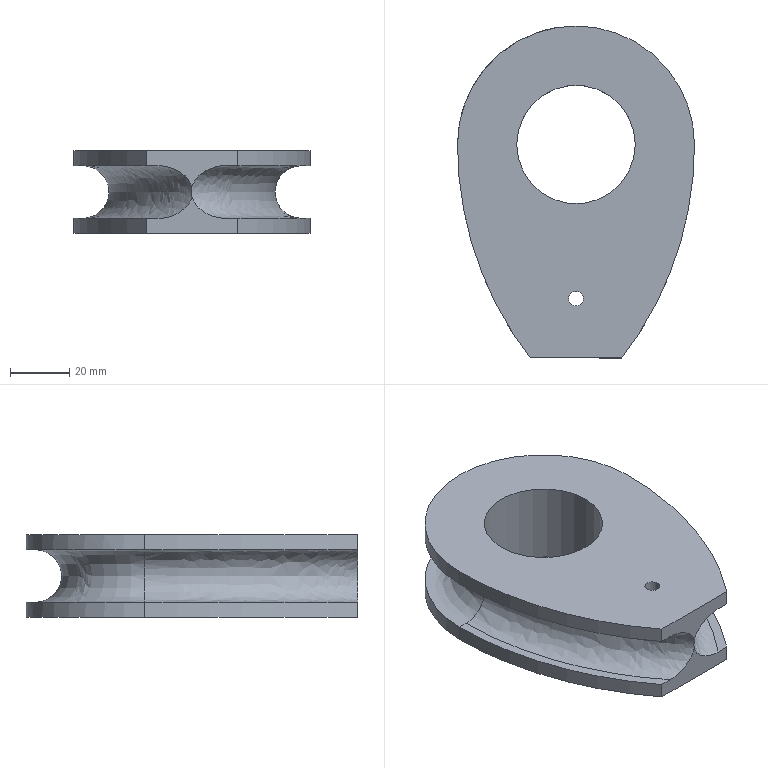Part | SolidWorks | features Extrusion 1, SweepCut 1 | 1 solid | 22 faces | box 80 x 112 x 28 mm | volume 116834 mm3 | cylinder 10 | plane 8 | spline 4 | commonest cylinder face diameters 236 x4 5 x2 40 x2 80 x2
STEP:
#1=CARTESIAN_POINT('',(-2.5,-52.,-14.));
#2=VERTEX_POINT('',#1);
#3=CARTESIAN_POINT('',(2.5,-52.,-14.));
#4=VERTEX_POINT('',#3);
#5=CARTESIAN_POINT('',(0.,-52.,-14.));
#6=DIRECTION('',(0.,0.,1.));
#7=DIRECTION('',(1.,0.,0.));
#8=AXIS2_PLACEMENT_3D('',#5,#6,#7);
#9=CIRCLE('',#8,2.5);
#10=EDGE_CURVE('',#2,#4,#9,.T.);
#11=ORIENTED_EDGE('',*,*,#10,.F.);
#12=CARTESIAN_POINT('',(-2.5,-52.,14.));
#13=VERTEX_POINT('',#12);
#14=CARTESIAN_POINT('',(-2.5,-52.,-14.));
#15=DIRECTION('',(0.,0.,1.));
#16=VECTOR('',#15,1000.);
#17=LINE('',#14,#16);
#18=EDGE_CURVE('',#2,#13,#17,.T.);
#19=ORIENTED_EDGE('',*,*,#18,.T.);
#20=CARTESIAN_POINT('',(2.5,-52.,14.));
#21=VERTEX_POINT('',#20);
#22=CARTESIAN_POINT('',(0.,-52.,14.));
#23=DIRECTION('',(0.,0.,1.));
#24=DIRECTION('',(1.,0.,0.));
#25=AXIS2_PLACEMENT_3D('',#22,#23,#24);
#26=CIRCLE('',#25,2.5);
#27=EDGE_CURVE('',#13,#21,#26,.T.);
#28=ORIENTED_EDGE('',*,*,#27,.T.);
#29=CARTESIAN_POINT('',(2.5,-52.,-14.));
#30=DIRECTION('',(0.,0.,1.));
#31=VECTOR('',#30,1000.);
#32=LINE('',#29,#31);
#33=EDGE_CURVE('',#4,#21,#32,.T.);
#34=ORIENTED_EDGE('',*,*,#33,.F.);
#35=EDGE_LOOP('',(#11,#19,#28,#34));
#36=FACE_OUTER_BOUND('',#35,.T.);
#37=CARTESIAN_POINT('',(0.,-52.,-14.));
#38=DIRECTION('',(0.,0.,1.));
#39=DIRECTION('',(1.,0.,0.));
#40=AXIS2_PLACEMENT_3D('',#37,#38,#39);
#41=CYLINDRICAL_SURFACE('',#40,2.5);
#42=ADVANCED_FACE('',(#36),#41,.F.);
#43=CARTESIAN_POINT('',(-20.,0.,-14.));
#44=VERTEX_POINT('',#43);
#45=CARTESIAN_POINT('',(20.,0.,-14.));
#46=VERTEX_POINT('',#45);
#47=CARTESIAN_POINT('',(0.,0.,-14.));
#48=DIRECTION('',(0.,0.,1.));
#49=DIRECTION('',(1.,0.,0.));
#50=AXIS2_PLACEMENT_3D('',#47,#48,#49);
#51=CIRCLE('',#50,20.);
#52=EDGE_CURVE('',#44,#46,#51,.T.);
#53=ORIENTED_EDGE('',*,*,#52,.F.);
#54=CARTESIAN_POINT('',(-20.,0.,14.));
#55=VERTEX_POINT('',#54);
#56=CARTESIAN_POINT('',(-20.,0.,-14.));
#57=DIRECTION('',(0.,0.,1.));
#58=VECTOR('',#57,1000.);
#59=LINE('',#56,#58);
#60=EDGE_CURVE('',#44,#55,#59,.T.);
#61=ORIENTED_EDGE('',*,*,#60,.T.);
#62=CARTESIAN_POINT('',(20.,0.,14.));
#63=VERTEX_POINT('',#62);
#64=CARTESIAN_POINT('',(0.,0.,14.));
#65=DIRECTION('',(0.,0.,1.));
#66=DIRECTION('',(1.,0.,0.));
#67=AXIS2_PLACEMENT_3D('',#64,#65,#66);
#68=CIRCLE('',#67,20.);
#69=EDGE_CURVE('',#55,#63,#68,.T.);
#70=ORIENTED_EDGE('',*,*,#69,.T.);
#71=CARTESIAN_POINT('',(20.,0.,-14.));
#72=DIRECTION('',(0.,0.,1.));
#73=VECTOR('',#72,1000.);
#74=LINE('',#71,#73);
#75=EDGE_CURVE('',#46,#63,#74,.T.);
#76=ORIENTED_EDGE('',*,*,#75,.F.);
#77=EDGE_LOOP('',(#53,#61,#70,#76));
#78=FACE_OUTER_BOUND('',#77,.T.);
#79=CARTESIAN_POINT('',(0.,0.,-14.));
#80=DIRECTION('',(0.,0.,1.));
#81=DIRECTION('',(1.,0.,0.));
#82=AXIS2_PLACEMENT_3D('',#79,#80,#81);
#83=CYLINDRICAL_SURFACE('',#82,20.);
#84=ADVANCED_FACE('',(#78),#83,.F.);
#85=CARTESIAN_POINT('',(0.,40.,-8.9));
#86=VERTEX_POINT('',#85);
#87=CARTESIAN_POINT('',(-40.,0.,-8.9));
#88=VERTEX_POINT('',#87);
#89=CARTESIAN_POINT('',(0.,40.,-8.9));
#90=CARTESIAN_POINT('',(-2.641,40.,-8.9));
#91=CARTESIAN_POINT('',(-5.238,39.741,-8.9));
#92=CARTESIAN_POINT('',(-9.07,38.98,-8.9));
#93=CARTESIAN_POINT('',(-10.337,38.664,-8.9));
#94=CARTESIAN_POINT('',(-12.22,38.093,-8.9));
#95=CARTESIAN_POINT('',(-12.847,37.887,-8.9));
#96=CARTESIAN_POINT('',(-14.089,37.442,-8.9));
#97=CARTESIAN_POINT('',(-14.702,37.206,-8.9));
#98=CARTESIAN_POINT('',(-17.728,35.952,-8.9));
#99=CARTESIAN_POINT('',(-20.025,34.725,-8.9));
#100=CARTESIAN_POINT('',(-22.741,32.913,-8.9));
#101=CARTESIAN_POINT('',(-23.277,32.537,-8.9));
#102=CARTESIAN_POINT('',(-24.332,31.755,-8.9));
#103=CARTESIAN_POINT('',(-24.853,31.349,-8.9));
#104=CARTESIAN_POINT('',(-26.382,30.096,-8.9));
#105=CARTESIAN_POINT('',(-27.352,29.216,-8.9));
#106=CARTESIAN_POINT('',(-30.119,26.451,-8.9));
#107=CARTESIAN_POINT('',(-31.775,24.439,-8.9));
#108=CARTESIAN_POINT('',(-33.603,21.709,-8.9));
#109=CARTESIAN_POINT('',(-33.957,21.151,-8.9));
#110=CARTESIAN_POINT('',(-34.635,20.022,-8.9));
#111=CARTESIAN_POINT('',(-34.958,19.451,-8.9));
#112=CARTESIAN_POINT('',(-35.884,17.721,-8.9));
#113=CARTESIAN_POINT('',(-37.,15.364,-8.9));
#114=CARTESIAN_POINT('',(-37.881,12.911,-8.9));
#115=CARTESIAN_POINT('',(-38.453,11.035,-8.9));
#116=CARTESIAN_POINT('',(-38.629,10.404,-8.9));
#117=CARTESIAN_POINT('',(-38.95,9.128,-8.9));
#118=CARTESIAN_POINT('',(-39.096,8.483,-8.9));
#119=CARTESIAN_POINT('',(-39.741,5.253,-8.9));
#120=CARTESIAN_POINT('',(-40.,2.641,-8.9));
#121=CARTESIAN_POINT('',(-40.,0.,-8.9));
#122=B_SPLINE_CURVE_WITH_KNOTS('',3,(#89,#90,#91,#92,#93,#94,#95,#96,#97,#98,#99,#100,#101,#102,#103,#104,#105,#106,#107,#108,#109,#110,#111,#112,#113,#114,#115,#116,#117,#118,#119,#120,#121),.UNSPECIFIED.,.F.,.F.,(4,2,2,2,2,2,2,2,2,2,2,2,1,2,2,2,4),(0.,0.007811,0.01172,0.01367,0.01562,0.02343,0.02539,0.02734,0.03124,0.03905,0.04101,0.04296,0.04686,0.05077,0.05272,0.05468,0.06249),.UNSPECIFIED.);
#123=EDGE_CURVE('',#86,#88,#122,.T.);
#124=ORIENTED_EDGE('',*,*,#123,.F.);
#125=CARTESIAN_POINT('',(40.,0.,-8.9));
#126=VERTEX_POINT('',#125);
#127=CARTESIAN_POINT('',(0.,0.,-8.9));
#128=DIRECTION('',(0.,0.,1.));
#129=DIRECTION('',(-1.,0.,0.));
#130=AXIS2_PLACEMENT_3D('',#127,#128,#129);
#131=CIRCLE('',#130,40.);
#132=EDGE_CURVE('',#126,#86,#131,.T.);
#133=ORIENTED_EDGE('',*,*,#132,.F.);
#134=CARTESIAN_POINT('',(40.,0.,-14.));
#135=VERTEX_POINT('',#134);
#136=CARTESIAN_POINT('',(40.,0.,-14.));
#137=DIRECTION('',(0.,0.,1.));
#138=VECTOR('',#137,1000.);
#139=LINE('',#136,#138);
#140=EDGE_CURVE('',#135,#126,#139,.T.);
#141=ORIENTED_EDGE('',*,*,#140,.F.);
#142=CARTESIAN_POINT('',(-40.,0.,-14.));
#143=VERTEX_POINT('',#142);
#144=CARTESIAN_POINT('',(0.,0.,-14.));
#145=DIRECTION('',(0.,0.,1.));
#146=DIRECTION('',(1.,0.,0.));
#147=AXIS2_PLACEMENT_3D('',#144,#145,#146);
#148=CIRCLE('',#147,40.);
#149=EDGE_CURVE('',#135,#143,#148,.T.);
#150=ORIENTED_EDGE('',*,*,#149,.T.);
#151=CARTESIAN_POINT('',(-40.,0.,-14.));
#152=DIRECTION('',(0.,0.,1.));
#153=VECTOR('',#152,1000.);
#154=LINE('',#151,#153);
#155=EDGE_CURVE('',#143,#88,#154,.T.);
#156=ORIENTED_EDGE('',*,*,#155,.T.);
#157=EDGE_LOOP('',(#124,#133,#141,#150,#156));
#158=FACE_OUTER_BOUND('',#157,.T.);
#159=CARTESIAN_POINT('',(0.,0.,-14.));
#160=DIRECTION('',(0.,0.,1.));
#161=DIRECTION('',(1.,0.,0.));
#162=AXIS2_PLACEMENT_3D('',#159,#160,#161);
#163=CYLINDRICAL_SURFACE('',#162,40.);
#164=ADVANCED_FACE('',(#158),#163,.T.);
#165=CARTESIAN_POINT('',(15.488,-72.,-8.9));
#166=VERTEX_POINT('',#165);
#167=CARTESIAN_POINT('',(-78.,0.,-8.9));
#168=DIRECTION('',(0.,0.,1.));
#169=DIRECTION('',(-1.,0.,0.));
#170=AXIS2_PLACEMENT_3D('',#167,#168,#169);
#171=CIRCLE('',#170,118.);
#172=EDGE_CURVE('',#166,#126,#171,.T.);
#173=ORIENTED_EDGE('',*,*,#172,.F.);
#174=CARTESIAN_POINT('',(15.488,-72.,-14.));
#175=VERTEX_POINT('',#174);
#176=CARTESIAN_POINT('',(15.488,-72.,-14.));
#177=DIRECTION('',(0.,0.,1.));
#178=VECTOR('',#177,1000.);
#179=LINE('',#176,#178);
#180=EDGE_CURVE('',#175,#166,#179,.T.);
#181=ORIENTED_EDGE('',*,*,#180,.F.);
#182=CARTESIAN_POINT('',(-78.,0.,-14.));
#183=DIRECTION('',(0.,0.,1.));
#184=DIRECTION('',(1.,0.,0.));
#185=AXIS2_PLACEMENT_3D('',#182,#183,#184);
#186=CIRCLE('',#185,118.);
#187=EDGE_CURVE('',#175,#135,#186,.T.);
#188=ORIENTED_EDGE('',*,*,#187,.T.);
#189=ORIENTED_EDGE('',*,*,#140,.T.);
#190=EDGE_LOOP('',(#173,#181,#188,#189));
#191=FACE_OUTER_BOUND('',#190,.T.);
#192=CARTESIAN_POINT('',(-78.,0.,-14.));
#193=DIRECTION('',(0.,0.,1.));
#194=DIRECTION('',(1.,0.,0.));
#195=AXIS2_PLACEMENT_3D('',#192,#193,#194);
#196=CYLINDRICAL_SURFACE('',#195,118.);
#197=ADVANCED_FACE('',(#191),#196,.T.);
#198=CARTESIAN_POINT('',(-15.488,-72.,-8.9));
#199=VERTEX_POINT('',#198);
#200=CARTESIAN_POINT('',(-11.48,-72.,-8.9));
#201=VERTEX_POINT('',#200);
#202=CARTESIAN_POINT('',(-15.488,-72.,-8.9));
#203=DIRECTION('',(1.,0.,0.));
#204=VECTOR('',#203,1000.);
#205=LINE('',#202,#204);
#206=EDGE_CURVE('',#199,#201,#205,.T.);
#207=ORIENTED_EDGE('',*,*,#206,.F.);
#208=CARTESIAN_POINT('',(-15.488,-72.,-14.));
#209=VERTEX_POINT('',#208);
#210=CARTESIAN_POINT('',(-15.488,-72.,-14.));
#211=DIRECTION('',(0.,0.,1.));
#212=VECTOR('',#211,1000.);
#213=LINE('',#210,#212);
#214=EDGE_CURVE('',#209,#199,#213,.T.);
#215=ORIENTED_EDGE('',*,*,#214,.F.);
#216=CARTESIAN_POINT('',(-15.488,-72.,-14.));
#217=DIRECTION('',(1.,0.,0.));
#218=VECTOR('',#217,1000.);
#219=LINE('',#216,#218);
#220=EDGE_CURVE('',#209,#175,#219,.T.);
#221=ORIENTED_EDGE('',*,*,#220,.T.);
#222=ORIENTED_EDGE('',*,*,#180,.T.);
#223=CARTESIAN_POINT('',(11.4,-72.,-8.9));
#224=VERTEX_POINT('',#223);
#225=CARTESIAN_POINT('',(-15.488,-72.,-8.9));
#226=DIRECTION('',(1.,0.,0.));
#227=VECTOR('',#226,1000.);
#228=LINE('',#225,#227);
#229=EDGE_CURVE('',#224,#166,#228,.T.);
#230=ORIENTED_EDGE('',*,*,#229,.F.);
#231=CARTESIAN_POINT('',(0.,-72.,-1.631));
#232=VERTEX_POINT('',#231);
#233=CARTESIAN_POINT('',(0.,-72.,-1.631));
#234=CARTESIAN_POINT('',(0.1499,-72.,-2.223));
#235=CARTESIAN_POINT('',(0.3744,-72.,-2.78));
#236=CARTESIAN_POINT('',(0.9485,-72.,-3.836));
#237=CARTESIAN_POINT('',(1.303,-72.,-4.338));
#238=CARTESIAN_POINT('',(2.092,-72.,-5.25));
#239=CARTESIAN_POINT('',(2.53,-72.,-5.667));
#240=CARTESIAN_POINT('',(3.476,-72.,-6.429));
#241=CARTESIAN_POINT('',(3.974,-72.,-6.766));
#242=CARTESIAN_POINT('',(5.011,-72.,-7.367));
#243=CARTESIAN_POINT('',(5.551,-72.,-7.63));
#244=CARTESIAN_POINT('',(6.388,-72.,-7.973));
#245=CARTESIAN_POINT('',(6.673,-72.,-8.079));
#246=CARTESIAN_POINT('',(7.247,-72.,-8.271));
#247=CARTESIAN_POINT('',(7.535,-72.,-8.357));
#248=CARTESIAN_POINT('',(8.407,-72.,-8.588));
#249=CARTESIAN_POINT('',(8.995,-72.,-8.704));
#250=CARTESIAN_POINT('',(10.187,-72.,-8.86));
#251=CARTESIAN_POINT('',(10.794,-72.,-8.9));
#252=CARTESIAN_POINT('',(11.4,-72.,-8.9));
#253=B_SPLINE_CURVE_WITH_KNOTS('',3,(#233,#234,#235,#236,#237,#238,#239,#240,#241,#242,#243,#244,#245,#246,#247,#248,#249,#250,#251,#252),.UNSPECIFIED.,.F.,.F.,(4,2,2,2,2,2,2,2,2,4),(0.,0.0018,0.003599,0.005399,0.007198,0.008998,0.009898,0.0108,0.0126,0.0144),.UNSPECIFIED.);
#254=EDGE_CURVE('',#232,#224,#253,.T.);
#255=ORIENTED_EDGE('',*,*,#254,.F.);
#256=CARTESIAN_POINT('',(-11.48,-72.,-8.9));
#257=CARTESIAN_POINT('',(-10.26,-72.,-8.9));
#258=CARTESIAN_POINT('',(-9.063,-72.,-8.744));
#259=CARTESIAN_POINT('',(-7.303,-72.,-8.284));
#260=CARTESIAN_POINT('',(-6.722,-72.,-8.091));
#261=CARTESIAN_POINT('',(-5.604,-72.,-7.638));
#262=CARTESIAN_POINT('',(-5.063,-72.,-7.376));
#263=CARTESIAN_POINT('',(-4.02,-72.,-6.779));
#264=CARTESIAN_POINT('',(-3.517,-72.,-6.444));
#265=CARTESIAN_POINT('',(-2.56,-72.,-5.683));
#266=CARTESIAN_POINT('',(-2.117,-72.,-5.268));
#267=CARTESIAN_POINT('',(-1.519,-72.,-4.584));
#268=CARTESIAN_POINT('',(-1.331,-72.,-4.346));
#269=CARTESIAN_POINT('',(-0.9784,-72.,-3.847));
#270=CARTESIAN_POINT('',(-0.8151,-72.,-3.587));
#271=CARTESIAN_POINT('',(-0.3777,-72.,-2.788));
#272=CARTESIAN_POINT('',(-0.1509,-72.,-2.227));
#273=CARTESIAN_POINT('',(0.,-72.,-1.631));
#274=B_SPLINE_CURVE_WITH_KNOTS('',3,(#256,#257,#258,#259,#260,#261,#262,#263,#264,#265,#266,#267,#268,#269,#270,#271,#272,#273),.UNSPECIFIED.,.F.,.F.,(4,2,2,2,2,2,2,2,4),(0.,0.003619,0.005428,0.007238,0.009047,0.01086,0.01176,0.01267,0.01448),.UNSPECIFIED.);
#275=EDGE_CURVE('',#201,#232,#274,.T.);
#276=ORIENTED_EDGE('',*,*,#275,.F.);
#277=EDGE_LOOP('',(#207,#215,#221,#222,#230,#255,#276));
#278=FACE_OUTER_BOUND('',#277,.T.);
#279=CARTESIAN_POINT('',(-15.488,-72.,-14.));
#280=DIRECTION('',(0.,-1.,0.));
#281=DIRECTION('',(1.,0.,0.));
#282=AXIS2_PLACEMENT_3D('',#279,#280,#281);
#283=PLANE('',#282);
#284=ADVANCED_FACE('',(#278),#283,.T.);
#285=CARTESIAN_POINT('',(78.,0.,-8.9));
#286=DIRECTION('',(0.,0.,1.));
#287=DIRECTION('',(-1.,0.,0.));
#288=AXIS2_PLACEMENT_3D('',#285,#286,#287);
#289=CIRCLE('',#288,118.);
#290=EDGE_CURVE('',#88,#199,#289,.T.);
#291=ORIENTED_EDGE('',*,*,#290,.F.);
#292=ORIENTED_EDGE('',*,*,#155,.F.);
#293=CARTESIAN_POINT('',(78.,0.,-14.));
#294=DIRECTION('',(0.,0.,1.));
#295=DIRECTION('',(1.,0.,0.));
#296=AXIS2_PLACEMENT_3D('',#293,#294,#295);
#297=CIRCLE('',#296,118.);
#298=EDGE_CURVE('',#143,#209,#297,.T.);
#299=ORIENTED_EDGE('',*,*,#298,.T.);
#300=ORIENTED_EDGE('',*,*,#214,.T.);
#301=EDGE_LOOP('',(#291,#292,#299,#300));
#302=FACE_OUTER_BOUND('',#301,.T.);
#303=CARTESIAN_POINT('',(78.,0.,-14.));
#304=DIRECTION('',(0.,0.,1.));
#305=DIRECTION('',(1.,0.,0.));
#306=AXIS2_PLACEMENT_3D('',#303,#304,#305);
#307=CYLINDRICAL_SURFACE('',#306,118.);
#308=ADVANCED_FACE('',(#302),#307,.T.);
#309=CARTESIAN_POINT('',(-40.,0.,8.9));
#310=VERTEX_POINT('',#309);
#311=CARTESIAN_POINT('',(0.,40.,8.9));
#312=VERTEX_POINT('',#311);
#313=CARTESIAN_POINT('',(-40.,0.,8.9));
#314=CARTESIAN_POINT('',(-40.,2.641,8.9));
#315=CARTESIAN_POINT('',(-39.741,5.238,8.9));
#316=CARTESIAN_POINT('',(-38.98,9.07,8.9));
#317=CARTESIAN_POINT('',(-38.664,10.337,8.9));
#318=CARTESIAN_POINT('',(-38.093,12.22,8.9));
#319=CARTESIAN_POINT('',(-37.887,12.847,8.9));
#320=CARTESIAN_POINT('',(-37.442,14.089,8.9));
#321=CARTESIAN_POINT('',(-37.206,14.702,8.9));
#322=CARTESIAN_POINT('',(-35.952,17.728,8.9));
#323=CARTESIAN_POINT('',(-34.725,20.025,8.9));
#324=CARTESIAN_POINT('',(-32.913,22.741,8.9));
#325=CARTESIAN_POINT('',(-32.537,23.277,8.9));
#326=CARTESIAN_POINT('',(-31.755,24.332,8.9));
#327=CARTESIAN_POINT('',(-31.349,24.853,8.9));
#328=CARTESIAN_POINT('',(-30.096,26.382,8.9));
#329=CARTESIAN_POINT('',(-29.216,27.352,8.9));
#330=CARTESIAN_POINT('',(-26.451,30.119,8.9));
#331=CARTESIAN_POINT('',(-24.439,31.775,8.9));
#332=CARTESIAN_POINT('',(-21.709,33.603,8.9));
#333=CARTESIAN_POINT('',(-21.151,33.957,8.9));
#334=CARTESIAN_POINT('',(-20.022,34.635,8.9));
#335=CARTESIAN_POINT('',(-19.451,34.958,8.9));
#336=CARTESIAN_POINT('',(-17.721,35.884,8.9));
#337=CARTESIAN_POINT('',(-15.364,37.,8.9));
#338=CARTESIAN_POINT('',(-12.911,37.881,8.9));
#339=CARTESIAN_POINT('',(-11.035,38.453,8.9));
#340=CARTESIAN_POINT('',(-10.404,38.629,8.9));
#341=CARTESIAN_POINT('',(-9.128,38.95,8.9));
#342=CARTESIAN_POINT('',(-8.483,39.096,8.9));
#343=CARTESIAN_POINT('',(-5.253,39.741,8.9));
#344=CARTESIAN_POINT('',(-2.641,40.,8.9));
#345=CARTESIAN_POINT('',(0.,40.,8.9));
#346=B_SPLINE_CURVE_WITH_KNOTS('',3,(#313,#314,#315,#316,#317,#318,#319,#320,#321,#322,#323,#324,#325,#326,#327,#328,#329,#330,#331,#332,#333,#334,#335,#336,#337,#338,#339,#340,#341,#342,#343,#344,#345),.UNSPECIFIED.,.F.,.F.,(4,2,2,2,2,2,2,2,2,2,2,2,1,2,2,2,4),(0.,0.007811,0.01172,0.01367,0.01562,0.02343,0.02539,0.02734,0.03124,0.03905,0.04101,0.04296,0.04686,0.05077,0.05272,0.05468,0.06249),.UNSPECIFIED.);
#347=EDGE_CURVE('',#310,#312,#346,.T.);
#348=ORIENTED_EDGE('',*,*,#347,.F.);
#349=CARTESIAN_POINT('',(-40.,0.,14.));
#350=VERTEX_POINT('',#349);
#351=CARTESIAN_POINT('',(-40.,0.,-14.));
#352=DIRECTION('',(0.,0.,1.));
#353=VECTOR('',#352,1000.);
#354=LINE('',#351,#353);
#355=EDGE_CURVE('',#310,#350,#354,.T.);
#356=ORIENTED_EDGE('',*,*,#355,.T.);
#357=CARTESIAN_POINT('',(40.,0.,14.));
#358=VERTEX_POINT('',#357);
#359=CARTESIAN_POINT('',(0.,0.,14.));
#360=DIRECTION('',(0.,0.,1.));
#361=DIRECTION('',(1.,0.,0.));
#362=AXIS2_PLACEMENT_3D('',#359,#360,#361);
#363=CIRCLE('',#362,40.);
#364=EDGE_CURVE('',#358,#350,#363,.T.);
#365=ORIENTED_EDGE('',*,*,#364,.F.);
#366=CARTESIAN_POINT('',(40.,0.,8.9));
#367=VERTEX_POINT('',#366);
#368=CARTESIAN_POINT('',(40.,0.,-14.));
#369=DIRECTION('',(0.,0.,1.));
#370=VECTOR('',#369,1000.);
#371=LINE('',#368,#370);
#372=EDGE_CURVE('',#367,#358,#371,.T.);
#373=ORIENTED_EDGE('',*,*,#372,.F.);
#374=CARTESIAN_POINT('',(0.,0.,8.9));
#375=DIRECTION('',(0.,0.,-1.));
#376=DIRECTION('',(1.,0.,0.));
#377=AXIS2_PLACEMENT_3D('',#374,#375,#376);
#378=CIRCLE('',#377,40.);
#379=EDGE_CURVE('',#312,#367,#378,.T.);
#380=ORIENTED_EDGE('',*,*,#379,.F.);
#381=EDGE_LOOP('',(#348,#356,#365,#373,#380));
#382=FACE_OUTER_BOUND('',#381,.T.);
#383=CARTESIAN_POINT('',(0.,0.,-14.));
#384=DIRECTION('',(0.,0.,1.));
#385=DIRECTION('',(1.,0.,0.));
#386=AXIS2_PLACEMENT_3D('',#383,#384,#385);
#387=CYLINDRICAL_SURFACE('',#386,40.);
#388=ADVANCED_FACE('',(#382),#387,.T.);
#389=CARTESIAN_POINT('',(15.488,-72.,8.9));
#390=VERTEX_POINT('',#389);
#391=CARTESIAN_POINT('',(-78.,0.,8.9));
#392=DIRECTION('',(0.,0.,-1.));
#393=DIRECTION('',(1.,0.,0.));
#394=AXIS2_PLACEMENT_3D('',#391,#392,#393);
#395=CIRCLE('',#394,118.);
#396=EDGE_CURVE('',#367,#390,#395,.T.);
#397=ORIENTED_EDGE('',*,*,#396,.F.);
#398=ORIENTED_EDGE('',*,*,#372,.T.);
#399=CARTESIAN_POINT('',(15.488,-72.,14.));
#400=VERTEX_POINT('',#399);
#401=CARTESIAN_POINT('',(-78.,0.,14.));
#402=DIRECTION('',(0.,0.,1.));
#403=DIRECTION('',(1.,0.,0.));
#404=AXIS2_PLACEMENT_3D('',#401,#402,#403);
#405=CIRCLE('',#404,118.);
#406=EDGE_CURVE('',#400,#358,#405,.T.);
#407=ORIENTED_EDGE('',*,*,#406,.F.);
#408=CARTESIAN_POINT('',(15.488,-72.,-14.));
#409=DIRECTION('',(0.,0.,1.));
#410=VECTOR('',#409,1000.);
#411=LINE('',#408,#410);
#412=EDGE_CURVE('',#390,#400,#411,.T.);
#413=ORIENTED_EDGE('',*,*,#412,.F.);
#414=EDGE_LOOP('',(#397,#398,#407,#413));
#415=FACE_OUTER_BOUND('',#414,.T.);
#416=CARTESIAN_POINT('',(-78.,0.,-14.));
#417=DIRECTION('',(0.,0.,1.));
#418=DIRECTION('',(1.,0.,0.));
#419=AXIS2_PLACEMENT_3D('',#416,#417,#418);
#420=CYLINDRICAL_SURFACE('',#419,118.);
#421=ADVANCED_FACE('',(#415),#420,.T.);
#422=CARTESIAN_POINT('',(-11.48,-72.,8.9));
#423=VERTEX_POINT('',#422);
#424=CARTESIAN_POINT('',(-15.488,-72.,8.9));
#425=VERTEX_POINT('',#424);
#426=CARTESIAN_POINT('',(-15.488,-72.,8.9));
#427=DIRECTION('',(-1.,0.,0.));
#428=VECTOR('',#427,1000.);
#429=LINE('',#426,#428);
#430=EDGE_CURVE('',#423,#425,#429,.T.);
#431=ORIENTED_EDGE('',*,*,#430,.F.);
#432=CARTESIAN_POINT('',(0.,-72.,1.631));
#433=VERTEX_POINT('',#432);
#434=CARTESIAN_POINT('',(0.,-72.,1.631));
#435=CARTESIAN_POINT('',(-0.1507,-72.,2.226));
#436=CARTESIAN_POINT('',(-0.3767,-72.,2.785));
#437=CARTESIAN_POINT('',(-0.956,-72.,3.845));
#438=CARTESIAN_POINT('',(-1.314,-72.,4.349));
#439=CARTESIAN_POINT('',(-2.111,-72.,5.262));
#440=CARTESIAN_POINT('',(-2.554,-72.,5.678));
#441=CARTESIAN_POINT('',(-3.509,-72.,6.438));
#442=CARTESIAN_POINT('',(-4.012,-72.,6.774));
#443=CARTESIAN_POINT('',(-5.056,-72.,7.373));
#444=CARTESIAN_POINT('',(-5.599,-72.,7.635));
#445=CARTESIAN_POINT('',(-6.442,-72.,7.978));
#446=CARTESIAN_POINT('',(-6.729,-72.,8.083));
#447=CARTESIAN_POINT('',(-7.305,-72.,8.274));
#448=CARTESIAN_POINT('',(-7.596,-72.,8.36));
#449=CARTESIAN_POINT('',(-8.472,-72.,8.59));
#450=CARTESIAN_POINT('',(-9.063,-72.,8.705));
#451=CARTESIAN_POINT('',(-10.262,-72.,8.86));
#452=CARTESIAN_POINT('',(-10.871,-72.,8.9));
#453=CARTESIAN_POINT('',(-11.48,-72.,8.9));
#454=B_SPLINE_CURVE_WITH_KNOTS('',3,(#434,#435,#436,#437,#438,#439,#440,#441,#442,#443,#444,#445,#446,#447,#448,#449,#450,#451,#452,#453),.UNSPECIFIED.,.F.,.F.,(4,2,2,2,2,2,2,2,2,4),(0.,0.001808,0.003617,0.005425,0.007233,0.009042,0.009946,0.01085,0.01266,0.01447),.UNSPECIFIED.);
#455=EDGE_CURVE('',#433,#423,#454,.T.);
#456=ORIENTED_EDGE('',*,*,#455,.F.);
#457=CARTESIAN_POINT('',(11.4,-72.,8.9));
#458=VERTEX_POINT('',#457);
#459=CARTESIAN_POINT('',(11.4,-72.,8.9));
#460=CARTESIAN_POINT('',(10.186,-72.,8.9));
#461=CARTESIAN_POINT('',(8.995,-72.,8.743));
#462=CARTESIAN_POINT('',(7.536,-72.,8.357));
#463=CARTESIAN_POINT('',(7.244,-72.,8.27));
#464=CARTESIAN_POINT('',(6.671,-72.,8.078));
#465=CARTESIAN_POINT('',(6.388,-72.,7.973));
#466=CARTESIAN_POINT('',(5.555,-72.,7.632));
#467=CARTESIAN_POINT('',(5.018,-72.,7.37));
#468=CARTESIAN_POINT('',(3.982,-72.,6.771));
#469=CARTESIAN_POINT('',(3.482,-72.,6.433));
#470=CARTESIAN_POINT('',(2.534,-72.,5.671));
#471=CARTESIAN_POINT('',(2.097,-72.,5.256));
#472=CARTESIAN_POINT('',(1.505,-72.,4.573));
#473=CARTESIAN_POINT('',(1.319,-72.,4.335));
#474=CARTESIAN_POINT('',(0.9699,-72.,3.837));
#475=CARTESIAN_POINT('',(0.8085,-72.,3.578));
#476=CARTESIAN_POINT('',(0.3753,-72.,2.783));
#477=CARTESIAN_POINT('',(0.1501,-72.,2.224));
#478=CARTESIAN_POINT('',(0.,-72.,1.631));
#479=B_SPLINE_CURVE_WITH_KNOTS('',3,(#459,#460,#461,#462,#463,#464,#465,#466,#467,#468,#469,#470,#471,#472,#473,#474,#475,#476,#477,#478),.UNSPECIFIED.,.F.,.F.,(4,2,2,2,2,2,2,2,2,4),(0.,0.003602,0.004503,0.005403,0.007204,0.009006,0.01081,0.01171,0.01261,0.01441),.UNSPECIFIED.);
#480=EDGE_CURVE('',#458,#433,#479,.T.);
#481=ORIENTED_EDGE('',*,*,#480,.F.);
#482=CARTESIAN_POINT('',(-15.488,-72.,8.9));
#483=DIRECTION('',(-1.,0.,0.));
#484=VECTOR('',#483,1000.);
#485=LINE('',#482,#484);
#486=EDGE_CURVE('',#390,#458,#485,.T.);
#487=ORIENTED_EDGE('',*,*,#486,.F.);
#488=ORIENTED_EDGE('',*,*,#412,.T.);
#489=CARTESIAN_POINT('',(-15.488,-72.,14.));
#490=VERTEX_POINT('',#489);
#491=CARTESIAN_POINT('',(-15.488,-72.,14.));
#492=DIRECTION('',(1.,0.,0.));
#493=VECTOR('',#492,1000.);
#494=LINE('',#491,#493);
#495=EDGE_CURVE('',#490,#400,#494,.T.);
#496=ORIENTED_EDGE('',*,*,#495,.F.);
#497=CARTESIAN_POINT('',(-15.488,-72.,-14.));
#498=DIRECTION('',(0.,0.,1.));
#499=VECTOR('',#498,1000.);
#500=LINE('',#497,#499);
#501=EDGE_CURVE('',#425,#490,#500,.T.);
#502=ORIENTED_EDGE('',*,*,#501,.F.);
#503=EDGE_LOOP('',(#431,#456,#481,#487,#488,#496,#502));
#504=FACE_OUTER_BOUND('',#503,.T.);
#505=CARTESIAN_POINT('',(-15.488,-72.,-14.));
#506=DIRECTION('',(0.,-1.,0.));
#507=DIRECTION('',(1.,0.,0.));
#508=AXIS2_PLACEMENT_3D('',#505,#506,#507);
#509=PLANE('',#508);
#510=ADVANCED_FACE('',(#504),#509,.T.);
#511=CARTESIAN_POINT('',(78.,0.,8.9));
#512=DIRECTION('',(0.,0.,-1.));
#513=DIRECTION('',(1.,0.,0.));
#514=AXIS2_PLACEMENT_3D('',#511,#512,#513);
#515=CIRCLE('',#514,118.);
#516=EDGE_CURVE('',#425,#310,#515,.T.);
#517=ORIENTED_EDGE('',*,*,#516,.F.);
#518=ORIENTED_EDGE('',*,*,#501,.T.);
#519=CARTESIAN_POINT('',(78.,0.,14.));
#520=DIRECTION('',(0.,0.,1.));
#521=DIRECTION('',(1.,0.,0.));
#522=AXIS2_PLACEMENT_3D('',#519,#520,#521);
#523=CIRCLE('',#522,118.);
#524=EDGE_CURVE('',#350,#490,#523,.T.);
#525=ORIENTED_EDGE('',*,*,#524,.F.);
#526=ORIENTED_EDGE('',*,*,#355,.F.);
#527=EDGE_LOOP('',(#517,#518,#525,#526));
#528=FACE_OUTER_BOUND('',#527,.T.);
#529=CARTESIAN_POINT('',(78.,0.,-14.));
#530=DIRECTION('',(0.,0.,1.));
#531=DIRECTION('',(1.,0.,0.));
#532=AXIS2_PLACEMENT_3D('',#529,#530,#531);
#533=CYLINDRICAL_SURFACE('',#532,118.);
#534=ADVANCED_FACE('',(#528),#533,.T.);
#535=CARTESIAN_POINT('',(0.,-52.,-14.));
#536=DIRECTION('',(0.,0.,1.));
#537=DIRECTION('',(1.,0.,0.));
#538=AXIS2_PLACEMENT_3D('',#535,#536,#537);
#539=CIRCLE('',#538,2.5);
#540=EDGE_CURVE('',#4,#2,#539,.T.);
#541=ORIENTED_EDGE('',*,*,#540,.T.);
#542=ORIENTED_EDGE('',*,*,#10,.T.);
#543=EDGE_LOOP('',(#541,#542));
#544=FACE_BOUND('',#543,.T.);
#545=CARTESIAN_POINT('',(0.,0.,-14.));
#546=DIRECTION('',(0.,0.,1.));
#547=DIRECTION('',(1.,0.,0.));
#548=AXIS2_PLACEMENT_3D('',#545,#546,#547);
#549=CIRCLE('',#548,20.);
#550=EDGE_CURVE('',#46,#44,#549,.T.);
#551=ORIENTED_EDGE('',*,*,#550,.T.);
#552=ORIENTED_EDGE('',*,*,#52,.T.);
#553=EDGE_LOOP('',(#551,#552));
#554=FACE_BOUND('',#553,.T.);
#555=ORIENTED_EDGE('',*,*,#149,.F.);
#556=ORIENTED_EDGE('',*,*,#187,.F.);
#557=ORIENTED_EDGE('',*,*,#220,.F.);
#558=ORIENTED_EDGE('',*,*,#298,.F.);
#559=EDGE_LOOP('',(#555,#556,#557,#558));
#560=FACE_OUTER_BOUND('',#559,.T.);
#561=CARTESIAN_POINT('',(0.,0.,-14.));
#562=DIRECTION('',(0.,0.,1.));
#563=DIRECTION('',(1.,0.,0.));
#564=AXIS2_PLACEMENT_3D('',#561,#562,#563);
#565=PLANE('',#564);
#566=ADVANCED_FACE('',(#544,#554,#560),#565,.F.);
#567=CARTESIAN_POINT('',(0.,-52.,14.));
#568=DIRECTION('',(0.,0.,1.));
#569=DIRECTION('',(1.,0.,0.));
#570=AXIS2_PLACEMENT_3D('',#567,#568,#569);
#571=CIRCLE('',#570,2.5);
#572=EDGE_CURVE('',#21,#13,#571,.T.);
#573=ORIENTED_EDGE('',*,*,#572,.F.);
#574=ORIENTED_EDGE('',*,*,#27,.F.);
#575=EDGE_LOOP('',(#573,#574));
#576=FACE_BOUND('',#575,.T.);
#577=CARTESIAN_POINT('',(0.,0.,14.));
#578=DIRECTION('',(0.,0.,1.));
#579=DIRECTION('',(1.,0.,0.));
#580=AXIS2_PLACEMENT_3D('',#577,#578,#579);
#581=CIRCLE('',#580,20.);
#582=EDGE_CURVE('',#63,#55,#581,.T.);
#583=ORIENTED_EDGE('',*,*,#582,.F.);
#584=ORIENTED_EDGE('',*,*,#69,.F.);
#585=EDGE_LOOP('',(#583,#584));
#586=FACE_BOUND('',#585,.T.);
#587=ORIENTED_EDGE('',*,*,#364,.T.);
#588=ORIENTED_EDGE('',*,*,#524,.T.);
#589=ORIENTED_EDGE('',*,*,#495,.T.);
#590=ORIENTED_EDGE('',*,*,#406,.T.);
#591=EDGE_LOOP('',(#587,#588,#589,#590));
#592=FACE_OUTER_BOUND('',#591,.T.);
#593=CARTESIAN_POINT('',(0.,0.,14.));
#594=DIRECTION('',(0.,0.,1.));
#595=DIRECTION('',(1.,0.,0.));
#596=AXIS2_PLACEMENT_3D('',#593,#594,#595);
#597=PLANE('',#596);
#598=ADVANCED_FACE('',(#576,#586,#592),#597,.T.);
#599=ORIENTED_EDGE('',*,*,#60,.F.);
#600=ORIENTED_EDGE('',*,*,#550,.F.);
#601=ORIENTED_EDGE('',*,*,#75,.T.);
#602=ORIENTED_EDGE('',*,*,#582,.T.);
#603=EDGE_LOOP('',(#599,#600,#601,#602));
#604=FACE_OUTER_BOUND('',#603,.T.);
#605=CARTESIAN_POINT('',(0.,0.,-14.));
#606=DIRECTION('',(0.,0.,1.));
#607=DIRECTION('',(1.,0.,0.));
#608=AXIS2_PLACEMENT_3D('',#605,#606,#607);
#609=CYLINDRICAL_SURFACE('',#608,20.);
#610=ADVANCED_FACE('',(#604),#609,.F.);
#611=ORIENTED_EDGE('',*,*,#18,.F.);
#612=ORIENTED_EDGE('',*,*,#540,.F.);
#613=ORIENTED_EDGE('',*,*,#33,.T.);
#614=ORIENTED_EDGE('',*,*,#572,.T.);
#615=EDGE_LOOP('',(#611,#612,#613,#614));
#616=FACE_OUTER_BOUND('',#615,.T.);
#617=CARTESIAN_POINT('',(0.,-52.,-14.));
#618=DIRECTION('',(0.,0.,1.));
#619=DIRECTION('',(1.,0.,0.));
#620=AXIS2_PLACEMENT_3D('',#617,#618,#619);
#621=CYLINDRICAL_SURFACE('',#620,2.5);
#622=ADVANCED_FACE('',(#616),#621,.F.);
#623=ORIENTED_EDGE('',*,*,#132,.T.);
#624=CARTESIAN_POINT('',(0.,36.9,-8.9));
#625=VERTEX_POINT('',#624);
#626=CARTESIAN_POINT('',(0.,40.,-8.9));
#627=CARTESIAN_POINT('',(0.,38.967,-8.9));
#628=CARTESIAN_POINT('',(0.,37.933,-8.9));
#629=CARTESIAN_POINT('',(0.,36.9,-8.9));
#630=B_SPLINE_CURVE_WITH_KNOTS('',3,(#626,#627,#628,#629),.UNSPECIFIED.,.F.,.F.,(4,4),(0.4498,0.5),.UNSPECIFIED.);
#631=EDGE_CURVE('',#86,#625,#630,.T.);
#632=ORIENTED_EDGE('',*,*,#631,.T.);
#633=CARTESIAN_POINT('',(36.9,0.,-8.9));
#634=VERTEX_POINT('',#633);
#635=CARTESIAN_POINT('',(36.9,0.,-8.9));
#636=CARTESIAN_POINT('',(36.9,2.527,-8.9));
#637=CARTESIAN_POINT('',(36.353,7.765,-8.9));
#638=CARTESIAN_POINT('',(33.86,15.431,-8.9));
#639=CARTESIAN_POINT('',(29.525,22.663,-8.9));
#640=CARTESIAN_POINT('',(24.035,28.343,-8.9));
#641=CARTESIAN_POINT('',(18.,32.428,-8.9));
#642=CARTESIAN_POINT('',(12.092,35.059,-8.9));
#643=CARTESIAN_POINT('',(6.023,36.569,-8.9));
#644=CARTESIAN_POINT('',(1.973,36.9,-8.9));
#645=CARTESIAN_POINT('',(0.,36.9,-8.9));
#646=B_SPLINE_CURVE_WITH_KNOTS('',3,(#635,#636,#637,#638,#639,#640,#641,#642,#643,#644,#645),.UNSPECIFIED.,.F.,.F.,(4,1,1,1,1,1,1,1,4),(0.,0.131,0.2707,0.4154,0.5633,0.6777,0.7902,0.8977,1.),.UNSPECIFIED.);
#647=EDGE_CURVE('',#634,#625,#646,.T.);
#648=ORIENTED_EDGE('',*,*,#647,.F.);
#649=CARTESIAN_POINT('',(11.4,-72.,-8.9));
#650=CARTESIAN_POINT('',(14.688,-67.952,-8.9));
#651=CARTESIAN_POINT('',(22.038,-57.846,-8.9));
#652=CARTESIAN_POINT('',(30.961,-38.613,-8.9));
#653=CARTESIAN_POINT('',(35.866,-18.755,-8.9));
#654=CARTESIAN_POINT('',(36.9,-6.197,-8.9));
#655=CARTESIAN_POINT('',(36.9,0.,-8.9));
#656=B_SPLINE_CURVE_WITH_KNOTS('',3,(#649,#650,#651,#652,#653,#654,#655),.UNSPECIFIED.,.F.,.F.,(4,1,1,1,4),(0.1985,0.3785,0.6217,0.8125,1.),.UNSPECIFIED.);
#657=EDGE_CURVE('',#224,#634,#656,.T.);
#658=ORIENTED_EDGE('',*,*,#657,.F.);
#659=ORIENTED_EDGE('',*,*,#229,.T.);
#660=ORIENTED_EDGE('',*,*,#172,.T.);
#661=EDGE_LOOP('',(#623,#632,#648,#658,#659,#660));
#662=FACE_OUTER_BOUND('',#661,.T.);
#663=CARTESIAN_POINT('',(-50.,0.,-8.9));
#664=DIRECTION('',(0.,0.,-1.));
#665=DIRECTION('',(1.,0.,0.));
#666=AXIS2_PLACEMENT_3D('',#663,#664,#665);
#667=PLANE('',#666);
#668=ADVANCED_FACE('',(#662),#667,.F.);
#669=ORIENTED_EDGE('',*,*,#379,.T.);
#670=ORIENTED_EDGE('',*,*,#396,.T.);
#671=ORIENTED_EDGE('',*,*,#486,.T.);
#672=CARTESIAN_POINT('',(36.9,0.,8.9));
#673=VERTEX_POINT('',#672);
#674=CARTESIAN_POINT('',(11.4,-72.,8.9));
#675=CARTESIAN_POINT('',(14.688,-67.952,8.9));
#676=CARTESIAN_POINT('',(22.038,-57.846,8.9));
#677=CARTESIAN_POINT('',(30.961,-38.613,8.9));
#678=CARTESIAN_POINT('',(35.866,-18.755,8.9));
#679=CARTESIAN_POINT('',(36.9,-6.197,8.9));
#680=CARTESIAN_POINT('',(36.9,0.,8.9));
#681=B_SPLINE_CURVE_WITH_KNOTS('',3,(#674,#675,#676,#677,#678,#679,#680),.UNSPECIFIED.,.F.,.F.,(4,1,1,1,4),(0.1985,0.3785,0.6217,0.8125,1.),.UNSPECIFIED.);
#682=EDGE_CURVE('',#458,#673,#681,.T.);
#683=ORIENTED_EDGE('',*,*,#682,.T.);
#684=CARTESIAN_POINT('',(0.,36.9,8.9));
#685=VERTEX_POINT('',#684);
#686=CARTESIAN_POINT('',(36.9,0.,8.9));
#687=CARTESIAN_POINT('',(36.9,2.527,8.9));
#688=CARTESIAN_POINT('',(36.353,7.765,8.9));
#689=CARTESIAN_POINT('',(33.86,15.431,8.9));
#690=CARTESIAN_POINT('',(29.525,22.663,8.9));
#691=CARTESIAN_POINT('',(24.035,28.343,8.9));
#692=CARTESIAN_POINT('',(18.,32.428,8.9));
#693=CARTESIAN_POINT('',(12.092,35.059,8.9));
#694=CARTESIAN_POINT('',(6.023,36.569,8.9));
#695=CARTESIAN_POINT('',(1.973,36.9,8.9));
#696=CARTESIAN_POINT('',(0.,36.9,8.9));
#697=B_SPLINE_CURVE_WITH_KNOTS('',3,(#686,#687,#688,#689,#690,#691,#692,#693,#694,#695,#696),.UNSPECIFIED.,.F.,.F.,(4,1,1,1,1,1,1,1,4),(0.,0.131,0.2707,0.4154,0.5633,0.6777,0.7902,0.8977,1.),.UNSPECIFIED.);
#698=EDGE_CURVE('',#673,#685,#697,.T.);
#699=ORIENTED_EDGE('',*,*,#698,.T.);
#700=CARTESIAN_POINT('',(0.,43.45,8.9));
#701=DIRECTION('',(0.,1.,0.));
#702=VECTOR('',#701,1000.);
#703=LINE('',#700,#702);
#704=EDGE_CURVE('',#685,#312,#703,.T.);
#705=ORIENTED_EDGE('',*,*,#704,.T.);
#706=EDGE_LOOP('',(#669,#670,#671,#683,#699,#705));
#707=FACE_OUTER_BOUND('',#706,.T.);
#708=CARTESIAN_POINT('',(-36.9,0.,8.9));
#709=DIRECTION('',(0.,0.,1.));
#710=DIRECTION('',(-1.,0.,0.));
#711=AXIS2_PLACEMENT_3D('',#708,#709,#710);
#712=PLANE('',#711);
#713=ADVANCED_FACE('',(#707),#712,.F.);
#714=ORIENTED_EDGE('',*,*,#347,.T.);
#715=ORIENTED_EDGE('',*,*,#704,.F.);
#716=CARTESIAN_POINT('',(0.,36.9,0.));
#717=DIRECTION('',(-1.,0.,0.));
#718=DIRECTION('',(0.,-1.,0.));
#719=AXIS2_PLACEMENT_3D('',#716,#717,#718);
#720=CIRCLE('',#719,8.9);
#721=EDGE_CURVE('',#625,#685,#720,.T.);
#722=ORIENTED_EDGE('',*,*,#721,.F.);
#723=ORIENTED_EDGE('',*,*,#631,.F.);
#724=ORIENTED_EDGE('',*,*,#123,.T.);
#725=CARTESIAN_POINT('',(-36.9,0.,-8.9));
#726=VERTEX_POINT('',#725);
#727=CARTESIAN_POINT('',(-40.,0.,-8.9));
#728=CARTESIAN_POINT('',(-38.967,0.,-8.9));
#729=CARTESIAN_POINT('',(-37.933,0.,-8.9));
#730=CARTESIAN_POINT('',(-36.9,0.,-8.9));
#731=B_SPLINE_CURVE_WITH_KNOTS('',3,(#727,#728,#729,#730),.UNSPECIFIED.,.F.,.F.,(4,4),(0.4498,0.5),.UNSPECIFIED.);
#732=EDGE_CURVE('',#88,#726,#731,.T.);
#733=ORIENTED_EDGE('',*,*,#732,.T.);
#734=CARTESIAN_POINT('',(-36.9,0.,8.9));
#735=VERTEX_POINT('',#734);
#736=CARTESIAN_POINT('',(-36.9,0.,-8.9));
#737=CARTESIAN_POINT('',(-19.1,0.,-8.9));
#738=CARTESIAN_POINT('',(-19.1,0.,8.9));
#739=CARTESIAN_POINT('',(-36.9,0.,8.9));
#740=(BOUNDED_CURVE()B_SPLINE_CURVE(3,(#736,#737,#738,#739),.UNSPECIFIED.,.F.,.F.)B_SPLINE_CURVE_WITH_KNOTS((4,4),(0.5,0.788),.UNSPECIFIED.)CURVE()GEOMETRIC_REPRESENTATION_ITEM()RATIONAL_B_SPLINE_CURVE((1.,0.3333,0.3333,1.))REPRESENTATION_ITEM(''));
#741=EDGE_CURVE('',#726,#735,#740,.T.);
#742=ORIENTED_EDGE('',*,*,#741,.T.);
#743=CARTESIAN_POINT('',(-36.9,0.,8.9));
#744=CARTESIAN_POINT('',(-37.933,0.,8.9));
#745=CARTESIAN_POINT('',(-38.967,0.,8.9));
#746=CARTESIAN_POINT('',(-40.,0.,8.9));
#747=B_SPLINE_CURVE_WITH_KNOTS('',3,(#743,#744,#745,#746),.UNSPECIFIED.,.F.,.F.,(4,4),(0.788,0.8382),.UNSPECIFIED.);
#748=EDGE_CURVE('',#735,#310,#747,.T.);
#749=ORIENTED_EDGE('',*,*,#748,.T.);
#750=EDGE_LOOP('',(#714,#715,#722,#723,#724,#733,#742,#749));
#751=FACE_OUTER_BOUND('',#750,.T.);
#752=CARTESIAN_POINT('',(0.,50.,-8.9));
#753=CARTESIAN_POINT('',(-3.427,49.794,-8.9));
#754=CARTESIAN_POINT('',(-10.508,49.368,-8.9));
#755=CARTESIAN_POINT('',(-20.938,45.835,-8.9));
#756=CARTESIAN_POINT('',(-30.68,40.042,-8.9));
#757=CARTESIAN_POINT('',(-38.43,32.535,-8.9));
#758=CARTESIAN_POINT('',(-43.93,24.42,-8.9));
#759=CARTESIAN_POINT('',(-47.495,16.366,-8.9));
#760=CARTESIAN_POINT('',(-49.613,8.169,-8.9));
#761=CARTESIAN_POINT('',(-49.873,2.678,-8.9));
#762=CARTESIAN_POINT('',(-50.,0.,-8.9));
#763=CARTESIAN_POINT('',(0.,45.633,-8.9));
#764=CARTESIAN_POINT('',(-3.128,45.445,-8.9));
#765=CARTESIAN_POINT('',(-9.593,45.055,-8.9));
#766=CARTESIAN_POINT('',(-19.102,41.836,-8.9));
#767=CARTESIAN_POINT('',(-28.007,36.538,-8.9));
#768=CARTESIAN_POINT('',(-35.068,29.701,-8.9));
#769=CARTESIAN_POINT('',(-40.098,22.281,-8.9));
#770=CARTESIAN_POINT('',(-43.346,14.941,-8.9));
#771=CARTESIAN_POINT('',(-45.28,7.454,-8.9));
#772=CARTESIAN_POINT('',(-45.518,2.443,-8.9));
#773=CARTESIAN_POINT('',(-45.633,0.,-8.9));
#774=CARTESIAN_POINT('',(0.,41.267,-8.9));
#775=CARTESIAN_POINT('',(-2.83,41.096,-8.9));
#776=CARTESIAN_POINT('',(-8.678,40.742,-8.9));
#777=CARTESIAN_POINT('',(-17.267,37.837,-8.9));
#778=CARTESIAN_POINT('',(-25.335,33.035,-8.9));
#779=CARTESIAN_POINT('',(-31.705,26.868,-8.9));
#780=CARTESIAN_POINT('',(-36.265,20.141,-8.9));
#781=CARTESIAN_POINT('',(-39.196,13.517,-8.9));
#782=CARTESIAN_POINT('',(-40.947,6.738,-8.9));
#783=CARTESIAN_POINT('',(-41.162,2.209,-8.9));
#784=CARTESIAN_POINT('',(-41.267,0.,-8.9));
#785=CARTESIAN_POINT('',(0.,36.9,-8.9));
#786=CARTESIAN_POINT('',(-2.531,36.747,-8.9));
#787=CARTESIAN_POINT('',(-7.763,36.429,-8.9));
#788=CARTESIAN_POINT('',(-15.431,33.838,-8.9));
#789=CARTESIAN_POINT('',(-22.663,29.531,-8.9));
#790=CARTESIAN_POINT('',(-28.342,24.034,-8.9));
#791=CARTESIAN_POINT('',(-32.432,18.001,-8.9));
#792=CARTESIAN_POINT('',(-35.046,12.092,-8.9));
#793=CARTESIAN_POINT('',(-36.615,6.023,-8.9));
#794=CARTESIAN_POINT('',(-36.806,1.974,-8.9));
#795=CARTESIAN_POINT('',(-36.9,0.,-8.9));
#796=CARTESIAN_POINT('',(0.,19.1,-8.9));
#797=CARTESIAN_POINT('',(-1.315,19.018,-8.9));
#798=CARTESIAN_POINT('',(-4.033,18.848,-8.9));
#799=CARTESIAN_POINT('',(-7.949,17.537,-8.9));
#800=CARTESIAN_POINT('',(-11.77,15.25,-8.9));
#801=CARTESIAN_POINT('',(-14.634,12.484,-8.9));
#802=CARTESIAN_POINT('',(-16.807,9.277,-8.9));
#803=CARTESIAN_POINT('',(-18.131,6.285,-8.9));
#804=CARTESIAN_POINT('',(-18.953,3.106,-8.9));
#805=CARTESIAN_POINT('',(-19.052,1.018,-8.9));
#806=CARTESIAN_POINT('',(-19.1,0.,-8.9));
#807=CARTESIAN_POINT('',(0.,19.1,8.9));
#808=CARTESIAN_POINT('',(-1.315,19.018,8.9));
#809=CARTESIAN_POINT('',(-4.033,18.848,8.9));
#810=CARTESIAN_POINT('',(-7.949,17.537,8.9));
#811=CARTESIAN_POINT('',(-11.77,15.25,8.9));
#812=CARTESIAN_POINT('',(-14.634,12.484,8.9));
#813=CARTESIAN_POINT('',(-16.807,9.277,8.9));
#814=CARTESIAN_POINT('',(-18.131,6.285,8.9));
#815=CARTESIAN_POINT('',(-18.953,3.106,8.9));
#816=CARTESIAN_POINT('',(-19.052,1.018,8.9));
#817=CARTESIAN_POINT('',(-19.1,0.,8.9));
#818=CARTESIAN_POINT('',(0.,36.9,8.9));
#819=CARTESIAN_POINT('',(-2.531,36.747,8.9));
#820=CARTESIAN_POINT('',(-7.763,36.429,8.9));
#821=CARTESIAN_POINT('',(-15.431,33.838,8.9));
#822=CARTESIAN_POINT('',(-22.663,29.531,8.9));
#823=CARTESIAN_POINT('',(-28.342,24.034,8.9));
#824=CARTESIAN_POINT('',(-32.432,18.001,8.9));
#825=CARTESIAN_POINT('',(-35.046,12.092,8.9));
#826=CARTESIAN_POINT('',(-36.615,6.023,8.9));
#827=CARTESIAN_POINT('',(-36.806,1.974,8.9));
#828=CARTESIAN_POINT('',(-36.9,0.,8.9));
#829=CARTESIAN_POINT('',(0.,41.267,8.9));
#830=CARTESIAN_POINT('',(-2.83,41.096,8.9));
#831=CARTESIAN_POINT('',(-8.678,40.742,8.9));
#832=CARTESIAN_POINT('',(-17.267,37.837,8.9));
#833=CARTESIAN_POINT('',(-25.335,33.035,8.9));
#834=CARTESIAN_POINT('',(-31.705,26.868,8.9));
#835=CARTESIAN_POINT('',(-36.265,20.141,8.9));
#836=CARTESIAN_POINT('',(-39.196,13.517,8.9));
#837=CARTESIAN_POINT('',(-40.947,6.738,8.9));
#838=CARTESIAN_POINT('',(-41.162,2.209,8.9));
#839=CARTESIAN_POINT('',(-41.267,0.,8.9));
#840=CARTESIAN_POINT('',(0.,45.633,8.9));
#841=CARTESIAN_POINT('',(-3.128,45.445,8.9));
#842=CARTESIAN_POINT('',(-9.593,45.055,8.9));
#843=CARTESIAN_POINT('',(-19.102,41.836,8.9));
#844=CARTESIAN_POINT('',(-28.007,36.538,8.9));
#845=CARTESIAN_POINT('',(-35.068,29.701,8.9));
#846=CARTESIAN_POINT('',(-40.098,22.281,8.9));
#847=CARTESIAN_POINT('',(-43.346,14.941,8.9));
#848=CARTESIAN_POINT('',(-45.28,7.454,8.9));
#849=CARTESIAN_POINT('',(-45.518,2.443,8.9));
#850=CARTESIAN_POINT('',(-45.633,0.,8.9));
#851=CARTESIAN_POINT('',(0.,50.,8.9));
#852=CARTESIAN_POINT('',(-3.427,49.794,8.9));
#853=CARTESIAN_POINT('',(-10.508,49.368,8.9));
#854=CARTESIAN_POINT('',(-20.938,45.835,8.9));
#855=CARTESIAN_POINT('',(-30.68,40.042,8.9));
#856=CARTESIAN_POINT('',(-38.43,32.535,8.9));
#857=CARTESIAN_POINT('',(-43.93,24.42,8.9));
#858=CARTESIAN_POINT('',(-47.495,16.366,8.9));
#859=CARTESIAN_POINT('',(-49.613,8.169,8.9));
#860=CARTESIAN_POINT('',(-49.873,2.678,8.9));
#861=CARTESIAN_POINT('',(-50.,0.,8.9));
#862=(BOUNDED_SURFACE()B_SPLINE_SURFACE(3,3,((#752,#753,#754,#755,#756,#757,#758,#759,#760,#761,#762),(#763,#764,#765,#766,#767,#768,#769,#770,#771,#772,#773),(#774,#775,#776,#777,#778,#779,#780,#781,#782,#783,#784),(#785,#786,#787,#788,#789,#790,#791,#792,#793,#794,#795),(#796,#797,#798,#799,#800,#801,#802,#803,#804,#805,#806),(#807,#808,#809,#810,#811,#812,#813,#814,#815,#816,#817),(#818,#819,#820,#821,#822,#823,#824,#825,#826,#827,#828),(#829,#830,#831,#832,#833,#834,#835,#836,#837,#838,#839),(#840,#841,#842,#843,#844,#845,#846,#847,#848,#849,#850),(#851,#852,#853,#854,#855,#856,#857,#858,#859,#860,#861)),.UNSPECIFIED.,.F.,.F.,.F.)B_SPLINE_SURFACE_WITH_KNOTS((4,3,3,4),(4,1,1,1,1,1,1,1,4),(0.288,0.5,0.788,1.),(0.,0.131,0.2707,0.4154,0.5633,0.6777,0.7902,0.8977,1.),.UNSPECIFIED.)GEOMETRIC_REPRESENTATION_ITEM()RATIONAL_B_SPLINE_SURFACE(((1.,1.,1.,1.,1.,1.,1.,1.,1.,1.,1.),(1.,1.,1.,1.,1.,1.,1.,1.,1.,1.,1.),(1.,1.,1.,1.,1.,1.,1.,1.,1.,1.,1.),(1.,1.,1.,1.,1.,1.,1.,1.,1.,1.,1.),(0.3333,0.3333,0.3333,0.3333,0.3333,0.3333,0.3333,0.3333,0.3333,0.3333,0.3333),(0.3333,0.3333,0.3333,0.3333,0.3333,0.3333,0.3333,0.3333,0.3333,0.3333,0.3333),(1.,1.,1.,1.,1.,1.,1.,1.,1.,1.,1.),(1.,1.,1.,1.,1.,1.,1.,1.,1.,1.,1.),(1.,1.,1.,1.,1.,1.,1.,1.,1.,1.,1.),(1.,1.,1.,1.,1.,1.,1.,1.,1.,1.,1.)))REPRESENTATION_ITEM('')SURFACE());
#863=ADVANCED_FACE('',(#751),#862,.F.);
#864=ORIENTED_EDGE('',*,*,#206,.T.);
#865=CARTESIAN_POINT('',(-36.9,0.,-8.9));
#866=CARTESIAN_POINT('',(-36.9,-7.905,-8.9));
#867=CARTESIAN_POINT('',(-35.209,-23.95,-8.9));
#868=CARTESIAN_POINT('',(-28.471,-45.058,-8.9));
#869=CARTESIAN_POINT('',(-19.234,-61.875,-8.9));
#870=CARTESIAN_POINT('',(-13.702,-69.267,-8.9));
#871=CARTESIAN_POINT('',(-11.48,-72.,-8.9));
#872=B_SPLINE_CURVE_WITH_KNOTS('',3,(#865,#866,#867,#868,#869,#870,#871),.UNSPECIFIED.,.F.,.F.,(4,1,1,1,4),(0.,0.2391,0.4824,0.6731,0.7961),.UNSPECIFIED.);
#873=EDGE_CURVE('',#726,#201,#872,.T.);
#874=ORIENTED_EDGE('',*,*,#873,.F.);
#875=ORIENTED_EDGE('',*,*,#732,.F.);
#876=ORIENTED_EDGE('',*,*,#290,.T.);
#877=EDGE_LOOP('',(#864,#874,#875,#876));
#878=FACE_OUTER_BOUND('',#877,.T.);
#879=CARTESIAN_POINT('',(-50.,0.,-8.9));
#880=DIRECTION('',(0.,0.,-1.));
#881=DIRECTION('',(1.,0.,0.));
#882=AXIS2_PLACEMENT_3D('',#879,#880,#881);
#883=PLANE('',#882);
#884=ADVANCED_FACE('',(#878),#883,.F.);
#885=ORIENTED_EDGE('',*,*,#455,.T.);
#886=CARTESIAN_POINT('',(-36.9,0.,8.9));
#887=CARTESIAN_POINT('',(-36.9,-7.905,8.9));
#888=CARTESIAN_POINT('',(-35.209,-23.95,8.9));
#889=CARTESIAN_POINT('',(-28.471,-45.058,8.9));
#890=CARTESIAN_POINT('',(-19.234,-61.875,8.9));
#891=CARTESIAN_POINT('',(-13.702,-69.267,8.9));
#892=CARTESIAN_POINT('',(-11.48,-72.,8.9));
#893=B_SPLINE_CURVE_WITH_KNOTS('',3,(#886,#887,#888,#889,#890,#891,#892),.UNSPECIFIED.,.F.,.F.,(4,1,1,1,4),(0.,0.2391,0.4824,0.6731,0.7961),.UNSPECIFIED.);
#894=EDGE_CURVE('',#735,#423,#893,.T.);
#895=ORIENTED_EDGE('',*,*,#894,.F.);
#896=ORIENTED_EDGE('',*,*,#741,.F.);
#897=ORIENTED_EDGE('',*,*,#873,.T.);
#898=ORIENTED_EDGE('',*,*,#275,.T.);
#899=CARTESIAN_POINT('',(0.,-72.,-1.631));
#900=CARTESIAN_POINT('',(0.,-71.702,-0.5498));
#901=CARTESIAN_POINT('',(0.,-71.702,0.5498));
#902=CARTESIAN_POINT('',(0.,-72.,1.631));
#903=(BOUNDED_CURVE()B_SPLINE_CURVE(3,(#899,#900,#901,#902),.UNSPECIFIED.,.F.,.F.)B_SPLINE_CURVE_WITH_KNOTS((4,4),(0.6307,0.6573),.UNSPECIFIED.)CURVE()GEOMETRIC_REPRESENTATION_ITEM()RATIONAL_B_SPLINE_CURVE((0.5043,0.4986,0.4986,0.5043))REPRESENTATION_ITEM(''));
#904=EDGE_CURVE('',#232,#433,#903,.T.);
#905=ORIENTED_EDGE('',*,*,#904,.T.);
#906=EDGE_LOOP('',(#885,#895,#896,#897,#898,#905));
#907=FACE_OUTER_BOUND('',#906,.T.);
#908=CARTESIAN_POINT('',(-36.9,0.,-8.9));
#909=CARTESIAN_POINT('',(-36.9,-7.905,-8.9));
#910=CARTESIAN_POINT('',(-35.209,-23.95,-8.9));
#911=CARTESIAN_POINT('',(-28.471,-45.058,-8.9));
#912=CARTESIAN_POINT('',(-15.853,-68.03,-8.9));
#913=CARTESIAN_POINT('',(-6.375,-77.993,-8.9));
#914=CARTESIAN_POINT('',(0.,-84.921,-8.9));
#915=CARTESIAN_POINT('',(-19.1,0.,-8.9));
#916=CARTESIAN_POINT('',(-19.1,-7.574,-8.9));
#917=CARTESIAN_POINT('',(-17.414,-20.092,-8.9));
#918=CARTESIAN_POINT('',(-12.813,-37.255,-8.9));
#919=CARTESIAN_POINT('',(1.75,-60.781,-8.9));
#920=CARTESIAN_POINT('',(-5.021,-53.178,-8.9));
#921=CARTESIAN_POINT('',(0.,-58.634,-8.9));
#922=CARTESIAN_POINT('',(-19.1,0.,8.9));
#923=CARTESIAN_POINT('',(-19.1,-7.617,8.9));
#924=CARTESIAN_POINT('',(-17.41,-20.076,8.9));
#925=CARTESIAN_POINT('',(-12.825,-37.245,8.9));
#926=CARTESIAN_POINT('',(1.796,-60.829,8.9));
#927=CARTESIAN_POINT('',(-5.196,-52.987,8.9));
#928=CARTESIAN_POINT('',(0.,-58.634,8.9));
#929=CARTESIAN_POINT('',(-36.9,0.,8.9));
#930=CARTESIAN_POINT('',(-36.9,-7.905,8.9));
#931=CARTESIAN_POINT('',(-35.209,-23.95,8.9));
#932=CARTESIAN_POINT('',(-28.471,-45.058,8.9));
#933=CARTESIAN_POINT('',(-15.853,-68.03,8.9));
#934=CARTESIAN_POINT('',(-6.375,-77.993,8.9));
#935=CARTESIAN_POINT('',(0.,-84.921,8.9));
#936=(BOUNDED_SURFACE()B_SPLINE_SURFACE(3,3,((#908,#909,#910,#911,#912,#913,#914),(#915,#916,#917,#918,#919,#920,#921),(#922,#923,#924,#925,#926,#927,#928),(#929,#930,#931,#932,#933,#934,#935)),.UNSPECIFIED.,.F.,.F.,.F.)B_SPLINE_SURFACE_WITH_KNOTS((4,4),(4,1,1,1,4),(0.5,0.788),(0.,0.2391,0.4824,0.6731,1.),.UNSPECIFIED.)GEOMETRIC_REPRESENTATION_ITEM()RATIONAL_B_SPLINE_SURFACE(((1.,1.,1.,1.,1.,1.,1.),(0.3333,0.3333,0.3333,0.3333,0.3333,0.3333,0.3333),(0.3333,0.3333,0.3333,0.3333,0.3333,0.3333,0.3333),(1.,1.,1.,1.,1.,1.,1.)))REPRESENTATION_ITEM('')SURFACE());
#937=ADVANCED_FACE('',(#907),#936,.F.);
#938=ORIENTED_EDGE('',*,*,#430,.T.);
#939=ORIENTED_EDGE('',*,*,#516,.T.);
#940=ORIENTED_EDGE('',*,*,#748,.F.);
#941=ORIENTED_EDGE('',*,*,#894,.T.);
#942=EDGE_LOOP('',(#938,#939,#940,#941));
#943=FACE_OUTER_BOUND('',#942,.T.);
#944=CARTESIAN_POINT('',(-36.9,0.,8.9));
#945=DIRECTION('',(0.,0.,1.));
#946=DIRECTION('',(-1.,0.,0.));
#947=AXIS2_PLACEMENT_3D('',#944,#945,#946);
#948=PLANE('',#947);
#949=ADVANCED_FACE('',(#943),#948,.F.);
#950=ORIENTED_EDGE('',*,*,#254,.T.);
#951=ORIENTED_EDGE('',*,*,#657,.T.);
#952=CARTESIAN_POINT('',(36.9,0.,0.));
#953=DIRECTION('',(0.,1.,0.));
#954=DIRECTION('',(-1.,0.,0.));
#955=AXIS2_PLACEMENT_3D('',#952,#953,#954);
#956=CIRCLE('',#955,8.9);
#957=EDGE_CURVE('',#634,#673,#956,.T.);
#958=ORIENTED_EDGE('',*,*,#957,.T.);
#959=ORIENTED_EDGE('',*,*,#682,.F.);
#960=ORIENTED_EDGE('',*,*,#480,.T.);
#961=ORIENTED_EDGE('',*,*,#904,.F.);
#962=EDGE_LOOP('',(#950,#951,#958,#959,#960,#961));
#963=FACE_OUTER_BOUND('',#962,.T.);
#964=CARTESIAN_POINT('',(0.,-84.921,-8.9));
#965=CARTESIAN_POINT('',(7.527,-76.741,-8.9));
#966=CARTESIAN_POINT('',(19.152,-64.065,-8.9));
#967=CARTESIAN_POINT('',(30.961,-38.613,-8.9));
#968=CARTESIAN_POINT('',(35.866,-18.755,-8.9));
#969=CARTESIAN_POINT('',(36.9,-6.197,-8.9));
#970=CARTESIAN_POINT('',(36.9,0.,-8.9));
#971=CARTESIAN_POINT('',(0.,-58.634,-8.9));
#972=CARTESIAN_POINT('',(6.068,-52.04,-8.9));
#973=CARTESIAN_POINT('',(0.6041,-57.885,-8.9));
#974=CARTESIAN_POINT('',(14.66,-32.117,-8.9));
#975=CARTESIAN_POINT('',(18.081,-15.687,-8.9));
#976=CARTESIAN_POINT('',(19.1,-5.927,-8.9));
#977=CARTESIAN_POINT('',(19.1,0.,-8.9));
#978=CARTESIAN_POINT('',(0.,-58.634,8.9));
#979=CARTESIAN_POINT('',(6.293,-51.795,8.9));
#980=CARTESIAN_POINT('',(0.5372,-57.954,8.9));
#981=CARTESIAN_POINT('',(14.671,-32.112,8.9));
#982=CARTESIAN_POINT('',(18.078,-15.67,8.9));
#983=CARTESIAN_POINT('',(19.1,-5.969,8.9));
#984=CARTESIAN_POINT('',(19.1,0.,8.9));
#985=CARTESIAN_POINT('',(0.,-84.921,8.9));
#986=CARTESIAN_POINT('',(7.527,-76.741,8.9));
#987=CARTESIAN_POINT('',(19.152,-64.065,8.9));
#988=CARTESIAN_POINT('',(30.961,-38.613,8.9));
#989=CARTESIAN_POINT('',(35.866,-18.755,8.9));
#990=CARTESIAN_POINT('',(36.9,-6.197,8.9));
#991=CARTESIAN_POINT('',(36.9,0.,8.9));
#992=(BOUNDED_SURFACE()B_SPLINE_SURFACE(3,3,((#964,#965,#966,#967,#968,#969,#970),(#971,#972,#973,#974,#975,#976,#977),(#978,#979,#980,#981,#982,#983,#984),(#985,#986,#987,#988,#989,#990,#991)),.UNSPECIFIED.,.F.,.F.,.F.)B_SPLINE_SURFACE_WITH_KNOTS((4,4),(4,1,1,1,4),(0.4487,0.7663),(0.,0.3785,0.6217,0.8125,1.),.UNSPECIFIED.)GEOMETRIC_REPRESENTATION_ITEM()RATIONAL_B_SPLINE_SURFACE(((1.,1.,1.,1.,1.,1.,1.),(0.3333,0.3333,0.3333,0.3333,0.3333,0.3333,0.3333),(0.3333,0.3333,0.3333,0.3333,0.3333,0.3333,0.3333),(1.,1.,1.,1.,1.,1.,1.)))REPRESENTATION_ITEM('')SURFACE());
#993=ADVANCED_FACE('',(#963),#992,.F.);
#994=ORIENTED_EDGE('',*,*,#957,.F.);
#995=ORIENTED_EDGE('',*,*,#647,.T.);
#996=ORIENTED_EDGE('',*,*,#721,.T.);
#997=ORIENTED_EDGE('',*,*,#698,.F.);
#998=EDGE_LOOP('',(#994,#995,#996,#997));
#999=FACE_OUTER_BOUND('',#998,.T.);
#1000=CARTESIAN_POINT('',(36.9,0.,-8.9));
#1001=CARTESIAN_POINT('',(36.9,2.527,-8.9));
#1002=CARTESIAN_POINT('',(36.353,7.765,-8.9));
#1003=CARTESIAN_POINT('',(33.86,15.431,-8.9));
#1004=CARTESIAN_POINT('',(29.525,22.663,-8.9));
#1005=CARTESIAN_POINT('',(24.035,28.343,-8.9));
#1006=CARTESIAN_POINT('',(18.,32.428,-8.9));
#1007=CARTESIAN_POINT('',(12.092,35.059,-8.9));
#1008=CARTESIAN_POINT('',(6.023,36.569,-8.9));
#1009=CARTESIAN_POINT('',(1.973,36.9,-8.9));
#1010=CARTESIAN_POINT('',(0.,36.9,-8.9));
#1011=CARTESIAN_POINT('',(19.1,0.,-8.9));
#1012=CARTESIAN_POINT('',(19.1,2.198,-8.9));
#1013=CARTESIAN_POINT('',(18.807,3.596,-8.9));
#1014=CARTESIAN_POINT('',(17.549,8.074,-8.9));
#1015=CARTESIAN_POINT('',(15.243,11.734,-8.9));
#1016=CARTESIAN_POINT('',(12.494,14.642,-8.9));
#1017=CARTESIAN_POINT('',(9.25,16.804,-8.9));
#1018=CARTESIAN_POINT('',(6.382,18.138,-8.9));
#1019=CARTESIAN_POINT('',(2.766,18.93,-8.9));
#1020=CARTESIAN_POINT('',(1.716,19.1,-8.9));
#1021=CARTESIAN_POINT('',(0.,19.1,-8.9));
#1022=CARTESIAN_POINT('',(19.1,0.,8.9));
#1023=CARTESIAN_POINT('',(19.1,2.24,8.9));
#1024=CARTESIAN_POINT('',(18.807,3.575,8.9));
#1025=CARTESIAN_POINT('',(17.549,8.08,8.9));
#1026=CARTESIAN_POINT('',(15.243,11.733,8.9));
#1027=CARTESIAN_POINT('',(12.495,14.643,8.9));
#1028=CARTESIAN_POINT('',(9.249,16.804,8.9));
#1029=CARTESIAN_POINT('',(6.387,18.138,8.9));
#1030=CARTESIAN_POINT('',(2.75,18.93,8.9));
#1031=CARTESIAN_POINT('',(1.749,19.1,8.9));
#1032=CARTESIAN_POINT('',(0.,19.1,8.9));
#1033=CARTESIAN_POINT('',(36.9,0.,8.9));
#1034=CARTESIAN_POINT('',(36.9,2.527,8.9));
#1035=CARTESIAN_POINT('',(36.353,7.765,8.9));
#1036=CARTESIAN_POINT('',(33.86,15.431,8.9));
#1037=CARTESIAN_POINT('',(29.525,22.663,8.9));
#1038=CARTESIAN_POINT('',(24.035,28.343,8.9));
#1039=CARTESIAN_POINT('',(18.,32.428,8.9));
#1040=CARTESIAN_POINT('',(12.092,35.059,8.9));
#1041=CARTESIAN_POINT('',(6.023,36.569,8.9));
#1042=CARTESIAN_POINT('',(1.973,36.9,8.9));
#1043=CARTESIAN_POINT('',(0.,36.9,8.9));
#1044=(BOUNDED_SURFACE()B_SPLINE_SURFACE(3,3,((#1000,#1001,#1002,#1003,#1004,#1005,#1006,#1007,#1008,#1009,#1010),(#1011,#1012,#1013,#1014,#1015,#1016,#1017,#1018,#1019,#1020,#1021),(#1022,#1023,#1024,#1025,#1026,#1027,#1028,#1029,#1030,#1031,#1032),(#1033,#1034,#1035,#1036,#1037,#1038,#1039,#1040,#1041,#1042,#1043)),.UNSPECIFIED.,.F.,.F.,.F.)B_SPLINE_SURFACE_WITH_KNOTS((4,4),(4,1,1,1,1,1,1,1,4),(0.5,0.788),(0.,0.131,0.2707,0.4154,0.5633,0.6777,0.7902,0.8977,1.),.UNSPECIFIED.)GEOMETRIC_REPRESENTATION_ITEM()RATIONAL_B_SPLINE_SURFACE(((1.,1.,1.,1.,1.,1.,1.,1.,1.,1.,1.),(0.3333,0.3333,0.3333,0.3333,0.3333,0.3333,0.3333,0.3333,0.3333,0.3333,0.3333),(0.3333,0.3333,0.3333,0.3333,0.3333,0.3333,0.3333,0.3333,0.3333,0.3333,0.3333),(1.,1.,1.,1.,1.,1.,1.,1.,1.,1.,1.)))REPRESENTATION_ITEM('')SURFACE());
#1045=ADVANCED_FACE('',(#999),#1044,.F.);
#1046=CLOSED_SHELL('',(#42,#84,#164,#197,#284,#308,#388,#421,#510,#534,#566,#598,#610,#622,#668,#713,#863,#884,#937,#949,#993,#1045));
#1047=MANIFOLD_SOLID_BREP('',#1046);
#1048=CARTESIAN_POINT('',(0.,0.,0.));
#1049=DIRECTION('',(0.,0.,1.));
#1050=DIRECTION('',(1.,0.,0.));
#1051=AXIS2_PLACEMENT_3D('',#1048,#1049,#1050);
#1052=(LENGTH_UNIT()NAMED_UNIT(*)SI_UNIT(.MILLI.,.METRE.));
#1053=UNCERTAINTY_MEASURE_WITH_UNIT(LENGTH_MEASURE(0.00001),#1052,'','');
#1054=(NAMED_UNIT(*)PLANE_ANGLE_UNIT()SI_UNIT($,.RADIAN.));
#1055=(NAMED_UNIT(*)SI_UNIT($,.STERADIAN.)SOLID_ANGLE_UNIT());
#1056=(GEOMETRIC_REPRESENTATION_CONTEXT(3)GLOBAL_UNCERTAINTY_ASSIGNED_CONTEXT((#1053))GLOBAL_UNIT_ASSIGNED_CONTEXT((#1052,#1054,#1055))REPRESENTATION_CONTEXT('',''));
#1057=ADVANCED_BREP_SHAPE_REPRESENTATION('',(#1047,#1051),#1056);